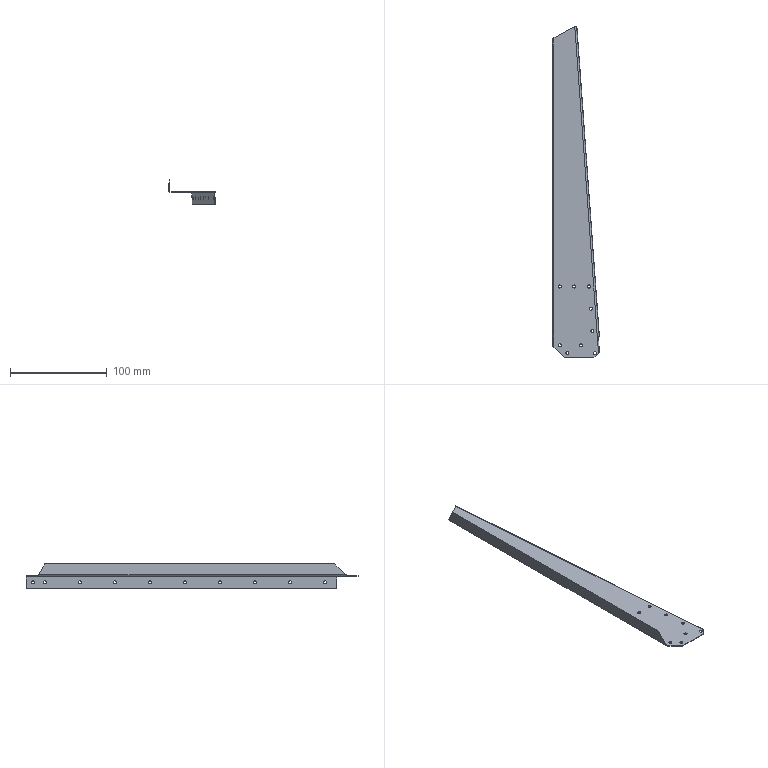Part | SolidWorks | features BaseBody 1 | 1 solid | 64 faces | box 48.56 x 343.706 x 25.097 mm | volume 9862 mm3 | cylinder 42 | plane 17 | spline 5 | commonest cylinder face diameters 3.2 x38 2 x2 3 x2